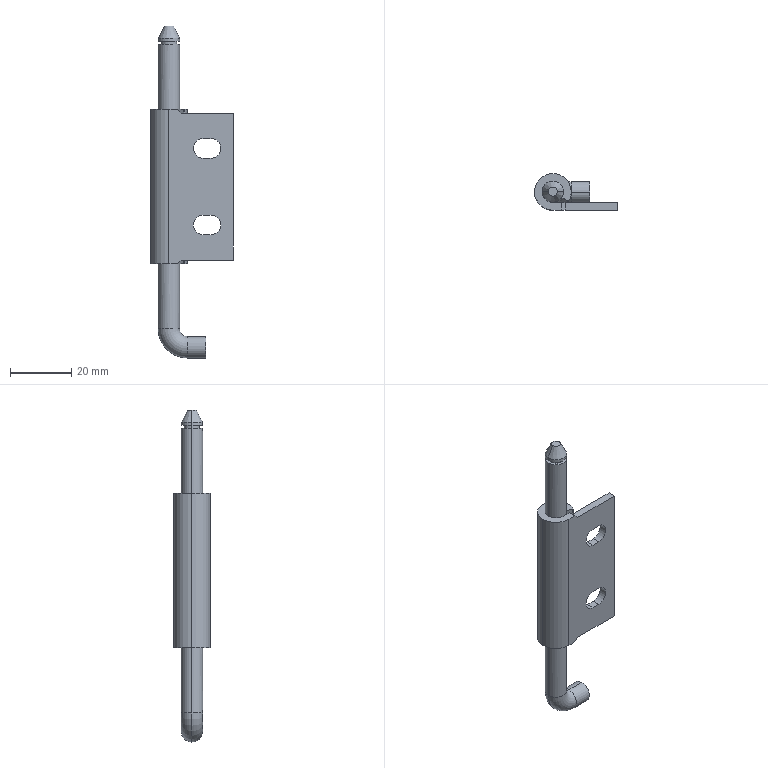Part | NX | features BREP 1 | 1 solid | 42 faces | box 27.1 x 12 x 108.5 mm | volume 9783 mm3 | plane 22 | cylinder 16 | cone 2 | torus 2 | commonest cylinder face diameters 7 x7 6.4 x4 12 x3 5 x2
STEP:
#1=CARTESIAN_POINT('',(-1.5,0.,52.5));
#2=VERTEX_POINT('',#1);
#3=CARTESIAN_POINT('',(1.5,0.,52.5));
#4=VERTEX_POINT('',#3);
#5=CARTESIAN_POINT('',(0.,0.,52.5));
#6=DIRECTION('',(0.,0.,-1.));
#7=DIRECTION('',(-1.,0.,0.));
#8=AXIS2_PLACEMENT_3D('',#5,#6,#7);
#9=CIRCLE('',#8,1.5);
#10=EDGE_CURVE('',#2,#4,#9,.T.);
#11=ORIENTED_EDGE('',*,*,#10,.F.);
#12=CARTESIAN_POINT('',(0.,0.,52.5));
#13=DIRECTION('',(0.,0.,-1.));
#14=DIRECTION('',(-1.,0.,0.));
#15=AXIS2_PLACEMENT_3D('',#12,#13,#14);
#16=CIRCLE('',#15,1.5);
#17=EDGE_CURVE('',#4,#2,#16,.T.);
#18=ORIENTED_EDGE('',*,*,#17,.F.);
#19=EDGE_LOOP('',(#11,#18));
#20=FACE_BOUND('',#19,.T.);
#21=CARTESIAN_POINT('',(0.,0.,52.5));
#22=DIRECTION('',(0.,0.,-1.));
#23=DIRECTION('',(-1.,0.,0.));
#24=AXIS2_PLACEMENT_3D('',#21,#22,#23);
#25=PLANE('',#24);
#26=ADVANCED_FACE('',(#20),#25,.F.);
#27=CARTESIAN_POINT('',(3.5,0.,48.5));
#28=VERTEX_POINT('',#27);
#29=CARTESIAN_POINT('',(1.5,0.,52.5));
#30=DIRECTION('',(0.4472,0.,-0.8944));
#31=VECTOR('',#30,1000.);
#32=LINE('',#29,#31);
#33=EDGE_CURVE('',#4,#28,#32,.T.);
#34=ORIENTED_EDGE('',*,*,#33,.F.);
#35=ORIENTED_EDGE('',*,*,#17,.T.);
#36=CARTESIAN_POINT('',(-3.5,0.,48.5));
#37=VERTEX_POINT('',#36);
#38=CARTESIAN_POINT('',(-1.5,0.,52.5));
#39=DIRECTION('',(-0.4472,0.,-0.8944));
#40=VECTOR('',#39,1000.);
#41=LINE('',#38,#40);
#42=EDGE_CURVE('',#2,#37,#41,.T.);
#43=ORIENTED_EDGE('',*,*,#42,.T.);
#44=CARTESIAN_POINT('',(0.,0.,48.5));
#45=DIRECTION('',(0.,0.,-1.));
#46=DIRECTION('',(-1.,0.,0.));
#47=AXIS2_PLACEMENT_3D('',#44,#45,#46);
#48=CIRCLE('',#47,3.5);
#49=EDGE_CURVE('',#28,#37,#48,.T.);
#50=ORIENTED_EDGE('',*,*,#49,.F.);
#51=EDGE_LOOP('',(#34,#35,#43,#50));
#52=FACE_BOUND('',#51,.T.);
#53=CARTESIAN_POINT('',(0.,0.,52.5));
#54=DIRECTION('',(0.,0.,-1.));
#55=DIRECTION('',(-1.,0.,0.));
#56=AXIS2_PLACEMENT_3D('',#53,#54,#55);
#57=CONICAL_SURFACE('',#56,1.5,0.4636);
#58=ADVANCED_FACE('',(#52),#57,.T.);
#59=CARTESIAN_POINT('',(3.5,0.,47.5));
#60=VERTEX_POINT('',#59);
#61=CARTESIAN_POINT('',(3.5,0.,-46.5));
#62=DIRECTION('',(0.,0.,-1.));
#63=VECTOR('',#62,1000.);
#64=LINE('',#61,#63);
#65=EDGE_CURVE('',#28,#60,#64,.T.);
#66=ORIENTED_EDGE('',*,*,#65,.F.);
#67=ORIENTED_EDGE('',*,*,#49,.T.);
#68=CARTESIAN_POINT('',(-3.5,0.,47.5));
#69=VERTEX_POINT('',#68);
#70=CARTESIAN_POINT('',(-3.5,0.,-46.5));
#71=DIRECTION('',(0.,0.,-1.));
#72=VECTOR('',#71,1000.);
#73=LINE('',#70,#72);
#74=EDGE_CURVE('',#37,#69,#73,.T.);
#75=ORIENTED_EDGE('',*,*,#74,.T.);
#76=CARTESIAN_POINT('',(0.,0.,47.5));
#77=DIRECTION('',(0.,0.,-1.));
#78=DIRECTION('',(-1.,0.,0.));
#79=AXIS2_PLACEMENT_3D('',#76,#77,#78);
#80=CIRCLE('',#79,3.5);
#81=EDGE_CURVE('',#60,#69,#80,.T.);
#82=ORIENTED_EDGE('',*,*,#81,.F.);
#83=EDGE_LOOP('',(#66,#67,#75,#82));
#84=FACE_BOUND('',#83,.T.);
#85=CARTESIAN_POINT('',(0.,0.,-46.5));
#86=DIRECTION('',(0.,0.,-1.));
#87=DIRECTION('',(-1.,0.,0.));
#88=AXIS2_PLACEMENT_3D('',#85,#86,#87);
#89=CYLINDRICAL_SURFACE('',#88,3.5);
#90=ADVANCED_FACE('',(#84),#89,.T.);
#91=CARTESIAN_POINT('',(0.,0.,47.5));
#92=DIRECTION('',(0.,0.,-1.));
#93=DIRECTION('',(-1.,0.,0.));
#94=AXIS2_PLACEMENT_3D('',#91,#92,#93);
#95=CIRCLE('',#94,3.5);
#96=EDGE_CURVE('',#69,#60,#95,.T.);
#97=ORIENTED_EDGE('',*,*,#96,.T.);
#98=ORIENTED_EDGE('',*,*,#81,.T.);
#99=EDGE_LOOP('',(#97,#98));
#100=FACE_BOUND('',#99,.T.);
#101=CARTESIAN_POINT('',(-2.5,0.,47.5));
#102=VERTEX_POINT('',#101);
#103=CARTESIAN_POINT('',(2.5,0.,47.5));
#104=VERTEX_POINT('',#103);
#105=CARTESIAN_POINT('',(0.,0.,47.5));
#106=DIRECTION('',(0.,0.,-1.));
#107=DIRECTION('',(-1.,0.,0.));
#108=AXIS2_PLACEMENT_3D('',#105,#106,#107);
#109=CIRCLE('',#108,2.5);
#110=EDGE_CURVE('',#102,#104,#109,.T.);
#111=ORIENTED_EDGE('',*,*,#110,.F.);
#112=CARTESIAN_POINT('',(0.,0.,47.5));
#113=DIRECTION('',(0.,0.,-1.));
#114=DIRECTION('',(-1.,0.,0.));
#115=AXIS2_PLACEMENT_3D('',#112,#113,#114);
#116=CIRCLE('',#115,2.5);
#117=EDGE_CURVE('',#104,#102,#116,.T.);
#118=ORIENTED_EDGE('',*,*,#117,.F.);
#119=EDGE_LOOP('',(#111,#118));
#120=FACE_BOUND('',#119,.T.);
#121=CARTESIAN_POINT('',(-3.5,0.,47.5));
#122=DIRECTION('',(0.,0.,1.));
#123=DIRECTION('',(1.,0.,0.));
#124=AXIS2_PLACEMENT_3D('',#121,#122,#123);
#125=PLANE('',#124);
#126=ADVANCED_FACE('',(#100,#120),#125,.F.);
#127=CARTESIAN_POINT('',(12.,0.,-49.));
#128=VERTEX_POINT('',#127);
#129=CARTESIAN_POINT('',(12.,0.,-56.));
#130=VERTEX_POINT('',#129);
#131=CARTESIAN_POINT('',(12.,0.,-52.5));
#132=DIRECTION('',(1.,0.,0.));
#133=DIRECTION('',(0.,0.,-1.));
#134=AXIS2_PLACEMENT_3D('',#131,#132,#133);
#135=CIRCLE('',#134,3.5);
#136=EDGE_CURVE('',#128,#130,#135,.T.);
#137=ORIENTED_EDGE('',*,*,#136,.T.);
#138=CARTESIAN_POINT('',(12.,0.,-52.5));
#139=DIRECTION('',(1.,0.,0.));
#140=DIRECTION('',(0.,0.,-1.));
#141=AXIS2_PLACEMENT_3D('',#138,#139,#140);
#142=CIRCLE('',#141,3.5);
#143=EDGE_CURVE('',#130,#128,#142,.T.);
#144=ORIENTED_EDGE('',*,*,#143,.T.);
#145=EDGE_LOOP('',(#137,#144));
#146=FACE_BOUND('',#145,.T.);
#147=CARTESIAN_POINT('',(12.,0.,-52.5));
#148=DIRECTION('',(1.,0.,0.));
#149=DIRECTION('',(0.,0.,-1.));
#150=AXIS2_PLACEMENT_3D('',#147,#148,#149);
#151=PLANE('',#150);
#152=ADVANCED_FACE('',(#146),#151,.T.);
#153=CARTESIAN_POINT('',(21.1,-6.,24.));
#154=VERTEX_POINT('',#153);
#155=CARTESIAN_POINT('',(21.1,-6.,-24.));
#156=VERTEX_POINT('',#155);
#157=CARTESIAN_POINT('',(21.1,-6.,24.));
#158=DIRECTION('',(0.,0.,-1.));
#159=VECTOR('',#158,1000.);
#160=LINE('',#157,#159);
#161=EDGE_CURVE('',#154,#156,#160,.T.);
#162=ORIENTED_EDGE('',*,*,#161,.T.);
#163=CARTESIAN_POINT('',(21.1,-3.5,-24.));
#164=VERTEX_POINT('',#163);
#165=CARTESIAN_POINT('',(21.1,-6.,-24.));
#166=DIRECTION('',(0.,1.,0.));
#167=VECTOR('',#166,1000.);
#168=LINE('',#165,#167);
#169=EDGE_CURVE('',#156,#164,#168,.T.);
#170=ORIENTED_EDGE('',*,*,#169,.T.);
#171=CARTESIAN_POINT('',(21.1,-3.5,24.));
#172=VERTEX_POINT('',#171);
#173=CARTESIAN_POINT('',(21.1,-3.5,24.));
#174=DIRECTION('',(0.,0.,-1.));
#175=VECTOR('',#174,1000.);
#176=LINE('',#173,#175);
#177=EDGE_CURVE('',#172,#164,#176,.T.);
#178=ORIENTED_EDGE('',*,*,#177,.F.);
#179=CARTESIAN_POINT('',(21.1,-3.5,24.));
#180=DIRECTION('',(0.,-1.,0.));
#181=VECTOR('',#180,1000.);
#182=LINE('',#179,#181);
#183=EDGE_CURVE('',#172,#154,#182,.T.);
#184=ORIENTED_EDGE('',*,*,#183,.T.);
#185=EDGE_LOOP('',(#162,#170,#178,#184));
#186=FACE_BOUND('',#185,.T.);
#187=CARTESIAN_POINT('',(21.1,-6.,25.25));
#188=DIRECTION('',(-1.,0.,0.));
#189=DIRECTION('',(0.,0.,1.));
#190=AXIS2_PLACEMENT_3D('',#187,#188,#189);
#191=PLANE('',#190);
#192=ADVANCED_FACE('',(#186),#191,.F.);
#193=ORIENTED_EDGE('',*,*,#183,.F.);
#194=CARTESIAN_POINT('',(4.,-3.5,24.));
#195=VERTEX_POINT('',#194);
#196=CARTESIAN_POINT('',(4.,-3.5,24.));
#197=DIRECTION('',(1.,0.,0.));
#198=VECTOR('',#197,1000.);
#199=LINE('',#196,#198);
#200=EDGE_CURVE('',#195,#172,#199,.T.);
#201=ORIENTED_EDGE('',*,*,#200,.F.);
#202=CARTESIAN_POINT('',(4.,-6.,24.));
#203=VERTEX_POINT('',#202);
#204=CARTESIAN_POINT('',(4.,-3.5,24.));
#205=DIRECTION('',(0.,-1.,0.));
#206=VECTOR('',#205,1000.);
#207=LINE('',#204,#206);
#208=EDGE_CURVE('',#195,#203,#207,.T.);
#209=ORIENTED_EDGE('',*,*,#208,.T.);
#210=CARTESIAN_POINT('',(21.1,-6.,24.));
#211=DIRECTION('',(-1.,0.,0.));
#212=VECTOR('',#211,1000.);
#213=LINE('',#210,#212);
#214=EDGE_CURVE('',#154,#203,#213,.T.);
#215=ORIENTED_EDGE('',*,*,#214,.F.);
#216=EDGE_LOOP('',(#193,#201,#209,#215));
#217=FACE_BOUND('',#216,.T.);
#218=CARTESIAN_POINT('',(4.,-3.,24.));
#219=DIRECTION('',(0.,0.,-1.));
#220=DIRECTION('',(-1.,0.,0.));
#221=AXIS2_PLACEMENT_3D('',#218,#219,#220);
#222=PLANE('',#221);
#223=ADVANCED_FACE('',(#217),#222,.F.);
#224=CARTESIAN_POINT('',(4.,-3.5,-24.));
#225=VERTEX_POINT('',#224);
#226=CARTESIAN_POINT('',(4.,-6.,-24.));
#227=VERTEX_POINT('',#226);
#228=CARTESIAN_POINT('',(4.,-3.5,-24.));
#229=DIRECTION('',(0.,-1.,0.));
#230=VECTOR('',#229,1000.);
#231=LINE('',#228,#230);
#232=EDGE_CURVE('',#225,#227,#231,.T.);
#233=ORIENTED_EDGE('',*,*,#232,.F.);
#234=CARTESIAN_POINT('',(21.1,-3.5,-24.));
#235=DIRECTION('',(-1.,0.,0.));
#236=VECTOR('',#235,1000.);
#237=LINE('',#234,#236);
#238=EDGE_CURVE('',#164,#225,#237,.T.);
#239=ORIENTED_EDGE('',*,*,#238,.F.);
#240=ORIENTED_EDGE('',*,*,#169,.F.);
#241=CARTESIAN_POINT('',(4.,-6.,-24.));
#242=DIRECTION('',(1.,0.,0.));
#243=VECTOR('',#242,1000.);
#244=LINE('',#241,#243);
#245=EDGE_CURVE('',#227,#156,#244,.T.);
#246=ORIENTED_EDGE('',*,*,#245,.F.);
#247=EDGE_LOOP('',(#233,#239,#240,#246));
#248=FACE_BOUND('',#247,.T.);
#249=CARTESIAN_POINT('',(22.9,-3.,-24.));
#250=DIRECTION('',(0.,0.,1.));
#251=DIRECTION('',(1.,0.,0.));
#252=AXIS2_PLACEMENT_3D('',#249,#250,#251);
#253=PLANE('',#252);
#254=ADVANCED_FACE('',(#248),#253,.F.);
#255=CARTESIAN_POINT('',(11.2,-6.,15.7));
#256=VERTEX_POINT('',#255);
#257=CARTESIAN_POINT('',(11.2,-6.,9.3));
#258=VERTEX_POINT('',#257);
#259=CARTESIAN_POINT('',(11.2,-6.,12.5));
#260=DIRECTION('',(0.,-1.,0.));
#261=DIRECTION('',(0.,0.,1.));
#262=AXIS2_PLACEMENT_3D('',#259,#260,#261);
#263=CIRCLE('',#262,3.2);
#264=EDGE_CURVE('',#256,#258,#263,.T.);
#265=ORIENTED_EDGE('',*,*,#264,.T.);
#266=CARTESIAN_POINT('',(11.2,-3.5,9.3));
#267=VERTEX_POINT('',#266);
#268=CARTESIAN_POINT('',(11.2,-3.5,9.3));
#269=DIRECTION('',(0.,-1.,0.));
#270=VECTOR('',#269,1000.);
#271=LINE('',#268,#270);
#272=EDGE_CURVE('',#267,#258,#271,.T.);
#273=ORIENTED_EDGE('',*,*,#272,.F.);
#274=CARTESIAN_POINT('',(11.2,-3.5,15.7));
#275=VERTEX_POINT('',#274);
#276=CARTESIAN_POINT('',(11.2,-3.5,12.5));
#277=DIRECTION('',(0.,1.,0.));
#278=DIRECTION('',(0.,0.,-1.));
#279=AXIS2_PLACEMENT_3D('',#276,#277,#278);
#280=CIRCLE('',#279,3.2);
#281=EDGE_CURVE('',#267,#275,#280,.T.);
#282=ORIENTED_EDGE('',*,*,#281,.T.);
#283=CARTESIAN_POINT('',(11.2,-3.5,15.7));
#284=DIRECTION('',(0.,-1.,0.));
#285=VECTOR('',#284,1000.);
#286=LINE('',#283,#285);
#287=EDGE_CURVE('',#275,#256,#286,.T.);
#288=ORIENTED_EDGE('',*,*,#287,.T.);
#289=EDGE_LOOP('',(#265,#273,#282,#288));
#290=FACE_BOUND('',#289,.T.);
#291=CARTESIAN_POINT('',(11.2,-3.,12.5));
#292=DIRECTION('',(0.,-1.,0.));
#293=DIRECTION('',(0.,0.,-1.));
#294=AXIS2_PLACEMENT_3D('',#291,#292,#293);
#295=CYLINDRICAL_SURFACE('',#294,3.2);
#296=ADVANCED_FACE('',(#290),#295,.F.);
#297=CARTESIAN_POINT('',(13.8,-6.,15.7));
#298=VERTEX_POINT('',#297);
#299=CARTESIAN_POINT('',(13.8,-6.,15.7));
#300=DIRECTION('',(-1.,0.,0.));
#301=VECTOR('',#300,1000.);
#302=LINE('',#299,#301);
#303=EDGE_CURVE('',#298,#256,#302,.T.);
#304=ORIENTED_EDGE('',*,*,#303,.T.);
#305=ORIENTED_EDGE('',*,*,#287,.F.);
#306=CARTESIAN_POINT('',(13.8,-3.5,15.7));
#307=VERTEX_POINT('',#306);
#308=CARTESIAN_POINT('',(11.2,-3.5,15.7));
#309=DIRECTION('',(1.,0.,0.));
#310=VECTOR('',#309,1000.);
#311=LINE('',#308,#310);
#312=EDGE_CURVE('',#275,#307,#311,.T.);
#313=ORIENTED_EDGE('',*,*,#312,.T.);
#314=CARTESIAN_POINT('',(13.8,-3.5,15.7));
#315=DIRECTION('',(0.,-1.,0.));
#316=VECTOR('',#315,1000.);
#317=LINE('',#314,#316);
#318=EDGE_CURVE('',#307,#298,#317,.T.);
#319=ORIENTED_EDGE('',*,*,#318,.T.);
#320=EDGE_LOOP('',(#304,#305,#313,#319));
#321=FACE_BOUND('',#320,.T.);
#322=CARTESIAN_POINT('',(11.2,-3.,15.7));
#323=DIRECTION('',(0.,0.,-1.));
#324=DIRECTION('',(-1.,0.,0.));
#325=AXIS2_PLACEMENT_3D('',#322,#323,#324);
#326=PLANE('',#325);
#327=ADVANCED_FACE('',(#321),#326,.T.);
#328=CARTESIAN_POINT('',(13.8,-6.,9.3));
#329=VERTEX_POINT('',#328);
#330=CARTESIAN_POINT('',(13.8,-6.,12.5));
#331=DIRECTION('',(0.,-1.,0.));
#332=DIRECTION('',(0.,0.,-1.));
#333=AXIS2_PLACEMENT_3D('',#330,#331,#332);
#334=CIRCLE('',#333,3.2);
#335=EDGE_CURVE('',#329,#298,#334,.T.);
#336=ORIENTED_EDGE('',*,*,#335,.T.);
#337=ORIENTED_EDGE('',*,*,#318,.F.);
#338=CARTESIAN_POINT('',(13.8,-3.5,9.3));
#339=VERTEX_POINT('',#338);
#340=CARTESIAN_POINT('',(13.8,-3.5,12.5));
#341=DIRECTION('',(0.,1.,0.));
#342=DIRECTION('',(0.,0.,1.));
#343=AXIS2_PLACEMENT_3D('',#340,#341,#342);
#344=CIRCLE('',#343,3.2);
#345=EDGE_CURVE('',#307,#339,#344,.T.);
#346=ORIENTED_EDGE('',*,*,#345,.T.);
#347=CARTESIAN_POINT('',(13.8,-3.5,9.3));
#348=DIRECTION('',(0.,-1.,0.));
#349=VECTOR('',#348,1000.);
#350=LINE('',#347,#349);
#351=EDGE_CURVE('',#339,#329,#350,.T.);
#352=ORIENTED_EDGE('',*,*,#351,.T.);
#353=EDGE_LOOP('',(#336,#337,#346,#352));
#354=FACE_BOUND('',#353,.T.);
#355=CARTESIAN_POINT('',(13.8,-3.,12.5));
#356=DIRECTION('',(0.,-1.,0.));
#357=DIRECTION('',(0.,0.,-1.));
#358=AXIS2_PLACEMENT_3D('',#355,#356,#357);
#359=CYLINDRICAL_SURFACE('',#358,3.2);
#360=ADVANCED_FACE('',(#354),#359,.F.);
#361=CARTESIAN_POINT('',(11.2,-6.,9.3));
#362=DIRECTION('',(1.,0.,0.));
#363=VECTOR('',#362,1000.);
#364=LINE('',#361,#363);
#365=EDGE_CURVE('',#258,#329,#364,.T.);
#366=ORIENTED_EDGE('',*,*,#365,.T.);
#367=ORIENTED_EDGE('',*,*,#351,.F.);
#368=CARTESIAN_POINT('',(13.8,-3.5,9.3));
#369=DIRECTION('',(-1.,0.,0.));
#370=VECTOR('',#369,1000.);
#371=LINE('',#368,#370);
#372=EDGE_CURVE('',#339,#267,#371,.T.);
#373=ORIENTED_EDGE('',*,*,#372,.T.);
#374=ORIENTED_EDGE('',*,*,#272,.T.);
#375=EDGE_LOOP('',(#366,#367,#373,#374));
#376=FACE_BOUND('',#375,.T.);
#377=CARTESIAN_POINT('',(13.8,-3.,9.3));
#378=DIRECTION('',(0.,0.,1.));
#379=DIRECTION('',(1.,0.,0.));
#380=AXIS2_PLACEMENT_3D('',#377,#378,#379);
#381=PLANE('',#380);
#382=ADVANCED_FACE('',(#376),#381,.T.);
#383=CARTESIAN_POINT('',(11.2,-6.,-9.3));
#384=VERTEX_POINT('',#383);
#385=CARTESIAN_POINT('',(11.2,-6.,-15.7));
#386=VERTEX_POINT('',#385);
#387=CARTESIAN_POINT('',(11.2,-6.,-12.5));
#388=DIRECTION('',(0.,-1.,0.));
#389=DIRECTION('',(0.,0.,1.));
#390=AXIS2_PLACEMENT_3D('',#387,#388,#389);
#391=CIRCLE('',#390,3.2);
#392=EDGE_CURVE('',#384,#386,#391,.T.);
#393=ORIENTED_EDGE('',*,*,#392,.T.);
#394=CARTESIAN_POINT('',(11.2,-3.5,-15.7));
#395=VERTEX_POINT('',#394);
#396=CARTESIAN_POINT('',(11.2,-3.5,-15.7));
#397=DIRECTION('',(0.,-1.,0.));
#398=VECTOR('',#397,1000.);
#399=LINE('',#396,#398);
#400=EDGE_CURVE('',#395,#386,#399,.T.);
#401=ORIENTED_EDGE('',*,*,#400,.F.);
#402=CARTESIAN_POINT('',(11.2,-3.5,-9.3));
#403=VERTEX_POINT('',#402);
#404=CARTESIAN_POINT('',(11.2,-3.5,-12.5));
#405=DIRECTION('',(0.,1.,0.));
#406=DIRECTION('',(0.,0.,-1.));
#407=AXIS2_PLACEMENT_3D('',#404,#405,#406);
#408=CIRCLE('',#407,3.2);
#409=EDGE_CURVE('',#395,#403,#408,.T.);
#410=ORIENTED_EDGE('',*,*,#409,.T.);
#411=CARTESIAN_POINT('',(11.2,-3.5,-9.3));
#412=DIRECTION('',(0.,-1.,0.));
#413=VECTOR('',#412,1000.);
#414=LINE('',#411,#413);
#415=EDGE_CURVE('',#403,#384,#414,.T.);
#416=ORIENTED_EDGE('',*,*,#415,.T.);
#417=EDGE_LOOP('',(#393,#401,#410,#416));
#418=FACE_BOUND('',#417,.T.);
#419=CARTESIAN_POINT('',(11.2,-3.,-12.5));
#420=DIRECTION('',(0.,-1.,0.));
#421=DIRECTION('',(0.,0.,-1.));
#422=AXIS2_PLACEMENT_3D('',#419,#420,#421);
#423=CYLINDRICAL_SURFACE('',#422,3.2);
#424=ADVANCED_FACE('',(#418),#423,.F.);
#425=CARTESIAN_POINT('',(13.8,-6.,-9.3));
#426=VERTEX_POINT('',#425);
#427=CARTESIAN_POINT('',(13.8,-6.,-9.3));
#428=DIRECTION('',(-1.,0.,0.));
#429=VECTOR('',#428,1000.);
#430=LINE('',#427,#429);
#431=EDGE_CURVE('',#426,#384,#430,.T.);
#432=ORIENTED_EDGE('',*,*,#431,.T.);
#433=ORIENTED_EDGE('',*,*,#415,.F.);
#434=CARTESIAN_POINT('',(13.8,-3.5,-9.3));
#435=VERTEX_POINT('',#434);
#436=CARTESIAN_POINT('',(11.2,-3.5,-9.3));
#437=DIRECTION('',(1.,0.,0.));
#438=VECTOR('',#437,1000.);
#439=LINE('',#436,#438);
#440=EDGE_CURVE('',#403,#435,#439,.T.);
#441=ORIENTED_EDGE('',*,*,#440,.T.);
#442=CARTESIAN_POINT('',(13.8,-3.5,-9.3));
#443=DIRECTION('',(0.,-1.,0.));
#444=VECTOR('',#443,1000.);
#445=LINE('',#442,#444);
#446=EDGE_CURVE('',#435,#426,#445,.T.);
#447=ORIENTED_EDGE('',*,*,#446,.T.);
#448=EDGE_LOOP('',(#432,#433,#441,#447));
#449=FACE_BOUND('',#448,.T.);
#450=CARTESIAN_POINT('',(11.2,-3.,-9.3));
#451=DIRECTION('',(0.,0.,-1.));
#452=DIRECTION('',(-1.,0.,0.));
#453=AXIS2_PLACEMENT_3D('',#450,#451,#452);
#454=PLANE('',#453);
#455=ADVANCED_FACE('',(#449),#454,.T.);
#456=CARTESIAN_POINT('',(13.8,-6.,-15.7));
#457=VERTEX_POINT('',#456);
#458=CARTESIAN_POINT('',(13.8,-6.,-12.5));
#459=DIRECTION('',(0.,-1.,0.));
#460=DIRECTION('',(0.,0.,-1.));
#461=AXIS2_PLACEMENT_3D('',#458,#459,#460);
#462=CIRCLE('',#461,3.2);
#463=EDGE_CURVE('',#457,#426,#462,.T.);
#464=ORIENTED_EDGE('',*,*,#463,.T.);
#465=ORIENTED_EDGE('',*,*,#446,.F.);
#466=CARTESIAN_POINT('',(13.8,-3.5,-15.7));
#467=VERTEX_POINT('',#466);
#468=CARTESIAN_POINT('',(13.8,-3.5,-12.5));
#469=DIRECTION('',(0.,1.,0.));
#470=DIRECTION('',(0.,0.,1.));
#471=AXIS2_PLACEMENT_3D('',#468,#469,#470);
#472=CIRCLE('',#471,3.2);
#473=EDGE_CURVE('',#435,#467,#472,.T.);
#474=ORIENTED_EDGE('',*,*,#473,.T.);
#475=CARTESIAN_POINT('',(13.8,-3.5,-15.7));
#476=DIRECTION('',(0.,-1.,0.));
#477=VECTOR('',#476,1000.);
#478=LINE('',#475,#477);
#479=EDGE_CURVE('',#467,#457,#478,.T.);
#480=ORIENTED_EDGE('',*,*,#479,.T.);
#481=EDGE_LOOP('',(#464,#465,#474,#480));
#482=FACE_BOUND('',#481,.T.);
#483=CARTESIAN_POINT('',(13.8,-3.,-12.5));
#484=DIRECTION('',(0.,-1.,0.));
#485=DIRECTION('',(0.,0.,-1.));
#486=AXIS2_PLACEMENT_3D('',#483,#484,#485);
#487=CYLINDRICAL_SURFACE('',#486,3.2);
#488=ADVANCED_FACE('',(#482),#487,.F.);
#489=CARTESIAN_POINT('',(11.2,-6.,-15.7));
#490=DIRECTION('',(1.,0.,0.));
#491=VECTOR('',#490,1000.);
#492=LINE('',#489,#491);
#493=EDGE_CURVE('',#386,#457,#492,.T.);
#494=ORIENTED_EDGE('',*,*,#493,.T.);
#495=ORIENTED_EDGE('',*,*,#479,.F.);
#496=CARTESIAN_POINT('',(13.8,-3.5,-15.7));
#497=DIRECTION('',(-1.,0.,0.));
#498=VECTOR('',#497,1000.);
#499=LINE('',#496,#498);
#500=EDGE_CURVE('',#467,#395,#499,.T.);
#501=ORIENTED_EDGE('',*,*,#500,.T.);
#502=ORIENTED_EDGE('',*,*,#400,.T.);
#503=EDGE_LOOP('',(#494,#495,#501,#502));
#504=FACE_BOUND('',#503,.T.);
#505=CARTESIAN_POINT('',(13.8,-3.,-15.7));
#506=DIRECTION('',(0.,0.,1.));
#507=DIRECTION('',(1.,0.,0.));
#508=AXIS2_PLACEMENT_3D('',#505,#506,#507);
#509=PLANE('',#508);
#510=ADVANCED_FACE('',(#504),#509,.T.);
#511=CARTESIAN_POINT('',(2.5,0.,46.5));
#512=VERTEX_POINT('',#511);
#513=CARTESIAN_POINT('',(2.5,0.,-46.5));
#514=DIRECTION('',(0.,0.,-1.));
#515=VECTOR('',#514,1000.);
#516=LINE('',#513,#515);
#517=EDGE_CURVE('',#104,#512,#516,.T.);
#518=ORIENTED_EDGE('',*,*,#517,.F.);
#519=ORIENTED_EDGE('',*,*,#117,.T.);
#520=CARTESIAN_POINT('',(-2.5,0.,46.5));
#521=VERTEX_POINT('',#520);
#522=CARTESIAN_POINT('',(-2.5,0.,-46.5));
#523=DIRECTION('',(0.,0.,-1.));
#524=VECTOR('',#523,1000.);
#525=LINE('',#522,#524);
#526=EDGE_CURVE('',#102,#521,#525,.T.);
#527=ORIENTED_EDGE('',*,*,#526,.T.);
#528=CARTESIAN_POINT('',(0.,0.,46.5));
#529=DIRECTION('',(0.,0.,-1.));
#530=DIRECTION('',(-1.,0.,0.));
#531=AXIS2_PLACEMENT_3D('',#528,#529,#530);
#532=CIRCLE('',#531,2.5);
#533=EDGE_CURVE('',#512,#521,#532,.T.);
#534=ORIENTED_EDGE('',*,*,#533,.F.);
#535=EDGE_LOOP('',(#518,#519,#527,#534));
#536=FACE_BOUND('',#535,.T.);
#537=CARTESIAN_POINT('',(0.,0.,-46.5));
#538=DIRECTION('',(0.,0.,-1.));
#539=DIRECTION('',(-1.,0.,0.));
#540=AXIS2_PLACEMENT_3D('',#537,#538,#539);
#541=CYLINDRICAL_SURFACE('',#540,2.5);
#542=ADVANCED_FACE('',(#536),#541,.T.);
#543=CARTESIAN_POINT('',(6.,0.,-56.));
#544=VERTEX_POINT('',#543);
#545=CARTESIAN_POINT('',(12.,0.,-56.));
#546=DIRECTION('',(-1.,0.,0.));
#547=VECTOR('',#546,1000.);
#548=LINE('',#545,#547);
#549=EDGE_CURVE('',#544,#130,#548,.F.);
#550=ORIENTED_EDGE('',*,*,#549,.T.);
#551=ORIENTED_EDGE('',*,*,#136,.F.);
#552=CARTESIAN_POINT('',(6.,0.,-49.));
#553=VERTEX_POINT('',#552);
#554=CARTESIAN_POINT('',(12.,0.,-49.));
#555=DIRECTION('',(-1.,0.,0.));
#556=VECTOR('',#555,1000.);
#557=LINE('',#554,#556);
#558=EDGE_CURVE('',#553,#128,#557,.F.);
#559=ORIENTED_EDGE('',*,*,#558,.F.);
#560=CARTESIAN_POINT('',(6.,0.,-52.5));
#561=DIRECTION('',(1.,0.,0.));
#562=DIRECTION('',(0.,0.,-1.));
#563=AXIS2_PLACEMENT_3D('',#560,#561,#562);
#564=CIRCLE('',#563,3.5);
#565=EDGE_CURVE('',#553,#544,#564,.T.);
#566=ORIENTED_EDGE('',*,*,#565,.T.);
#567=EDGE_LOOP('',(#550,#551,#559,#566));
#568=FACE_BOUND('',#567,.T.);
#569=CARTESIAN_POINT('',(12.,0.,-52.5));
#570=DIRECTION('',(-1.,0.,0.));
#571=DIRECTION('',(0.,0.,1.));
#572=AXIS2_PLACEMENT_3D('',#569,#570,#571);
#573=CYLINDRICAL_SURFACE('',#572,3.5);
#574=ADVANCED_FACE('',(#568),#573,.T.);
#575=ORIENTED_EDGE('',*,*,#208,.F.);
#576=CARTESIAN_POINT('',(2.75,-3.5,25.25));
#577=VERTEX_POINT('',#576);
#578=CARTESIAN_POINT('',(2.75,-3.5,25.25));
#579=DIRECTION('',(0.7071,0.,-0.7071));
#580=VECTOR('',#579,1000.);
#581=LINE('',#578,#580);
#582=EDGE_CURVE('',#577,#195,#581,.T.);
#583=ORIENTED_EDGE('',*,*,#582,.F.);
#584=CARTESIAN_POINT('',(2.75,-6.,25.25));
#585=VERTEX_POINT('',#584);
#586=CARTESIAN_POINT('',(2.75,-3.5,25.25));
#587=DIRECTION('',(0.,-1.,0.));
#588=VECTOR('',#587,1000.);
#589=LINE('',#586,#588);
#590=EDGE_CURVE('',#577,#585,#589,.T.);
#591=ORIENTED_EDGE('',*,*,#590,.T.);
#592=CARTESIAN_POINT('',(4.,-6.,24.));
#593=DIRECTION('',(-0.7071,0.,0.7071));
#594=VECTOR('',#593,1000.);
#595=LINE('',#592,#594);
#596=EDGE_CURVE('',#203,#585,#595,.T.);
#597=ORIENTED_EDGE('',*,*,#596,.F.);
#598=EDGE_LOOP('',(#575,#583,#591,#597));
#599=FACE_BOUND('',#598,.T.);
#600=CARTESIAN_POINT('',(2.75,-3.,25.25));
#601=DIRECTION('',(-0.7071,0.,-0.7071));
#602=DIRECTION('',(-0.7071,0.,0.7071));
#603=AXIS2_PLACEMENT_3D('',#600,#601,#602);
#604=PLANE('',#603);
#605=ADVANCED_FACE('',(#599),#604,.F.);
#606=CARTESIAN_POINT('',(0.,-6.,-25.25));
#607=VERTEX_POINT('',#606);
#608=CARTESIAN_POINT('',(2.75,-6.,-25.25));
#609=VERTEX_POINT('',#608);
#610=CARTESIAN_POINT('',(0.,-6.,-25.25));
#611=DIRECTION('',(1.,0.,0.));
#612=VECTOR('',#611,1000.);
#613=LINE('',#610,#612);
#614=EDGE_CURVE('',#607,#609,#613,.T.);
#615=ORIENTED_EDGE('',*,*,#614,.T.);
#616=CARTESIAN_POINT('',(2.75,-6.,-25.25));
#617=DIRECTION('',(0.7071,0.,0.7071));
#618=VECTOR('',#617,1000.);
#619=LINE('',#616,#618);
#620=EDGE_CURVE('',#609,#227,#619,.T.);
#621=ORIENTED_EDGE('',*,*,#620,.T.);
#622=ORIENTED_EDGE('',*,*,#245,.T.);
#623=ORIENTED_EDGE('',*,*,#161,.F.);
#624=ORIENTED_EDGE('',*,*,#214,.T.);
#625=ORIENTED_EDGE('',*,*,#596,.T.);
#626=CARTESIAN_POINT('',(0.,-6.,25.25));
#627=VERTEX_POINT('',#626);
#628=CARTESIAN_POINT('',(0.,-6.,25.25));
#629=DIRECTION('',(1.,0.,0.));
#630=VECTOR('',#629,1000.);
#631=LINE('',#628,#630);
#632=EDGE_CURVE('',#627,#585,#631,.T.);
#633=ORIENTED_EDGE('',*,*,#632,.F.);
#634=CARTESIAN_POINT('',(0.,-6.,25.25));
#635=DIRECTION('',(0.,0.,-1.));
#636=VECTOR('',#635,1000.);
#637=LINE('',#634,#636);
#638=EDGE_CURVE('',#627,#607,#637,.T.);
#639=ORIENTED_EDGE('',*,*,#638,.T.);
#640=EDGE_LOOP('',(#615,#621,#622,#623,#624,#625,#633,#639));
#641=FACE_BOUND('',#640,.T.);
#642=ORIENTED_EDGE('',*,*,#365,.F.);
#643=ORIENTED_EDGE('',*,*,#264,.F.);
#644=ORIENTED_EDGE('',*,*,#303,.F.);
#645=ORIENTED_EDGE('',*,*,#335,.F.);
#646=EDGE_LOOP('',(#642,#643,#644,#645));
#647=FACE_BOUND('',#646,.T.);
#648=ORIENTED_EDGE('',*,*,#493,.F.);
#649=ORIENTED_EDGE('',*,*,#392,.F.);
#650=ORIENTED_EDGE('',*,*,#431,.F.);
#651=ORIENTED_EDGE('',*,*,#463,.F.);
#652=EDGE_LOOP('',(#648,#649,#650,#651));
#653=FACE_BOUND('',#652,.T.);
#654=CARTESIAN_POINT('',(0.,-6.,25.25));
#655=DIRECTION('',(0.,1.,0.));
#656=DIRECTION('',(0.,0.,1.));
#657=AXIS2_PLACEMENT_3D('',#654,#655,#656);
#658=PLANE('',#657);
#659=ADVANCED_FACE('',(#641,#647,#653),#658,.F.);
#660=CARTESIAN_POINT('',(2.75,-3.5,-25.25));
#661=VERTEX_POINT('',#660);
#662=CARTESIAN_POINT('',(2.75,-3.5,-25.25));
#663=DIRECTION('',(0.,-1.,0.));
#664=VECTOR('',#663,1000.);
#665=LINE('',#662,#664);
#666=EDGE_CURVE('',#661,#609,#665,.T.);
#667=ORIENTED_EDGE('',*,*,#666,.F.);
#668=CARTESIAN_POINT('',(4.,-3.5,-24.));
#669=DIRECTION('',(-0.7071,0.,-0.7071));
#670=VECTOR('',#669,1000.);
#671=LINE('',#668,#670);
#672=EDGE_CURVE('',#225,#661,#671,.T.);
#673=ORIENTED_EDGE('',*,*,#672,.F.);
#674=ORIENTED_EDGE('',*,*,#232,.T.);
#675=ORIENTED_EDGE('',*,*,#620,.F.);
#676=EDGE_LOOP('',(#667,#673,#674,#675));
#677=FACE_BOUND('',#676,.T.);
#678=CARTESIAN_POINT('',(4.,-3.,-24.));
#679=DIRECTION('',(-0.7071,0.,0.7071));
#680=DIRECTION('',(0.7071,0.,0.7071));
#681=AXIS2_PLACEMENT_3D('',#678,#679,#680);
#682=PLANE('',#681);
#683=ADVANCED_FACE('',(#677),#682,.F.);
#684=ORIENTED_EDGE('',*,*,#238,.T.);
#685=ORIENTED_EDGE('',*,*,#672,.T.);
#686=CARTESIAN_POINT('',(0.,-3.5,-25.25));
#687=VERTEX_POINT('',#686);
#688=CARTESIAN_POINT('',(2.75,-3.5,-25.25));
#689=DIRECTION('',(-1.,0.,0.));
#690=VECTOR('',#689,1000.);
#691=LINE('',#688,#690);
#692=EDGE_CURVE('',#661,#687,#691,.T.);
#693=ORIENTED_EDGE('',*,*,#692,.T.);
#694=CARTESIAN_POINT('',(0.,-3.5,25.25));
#695=VERTEX_POINT('',#694);
#696=CARTESIAN_POINT('',(0.,-3.5,25.25));
#697=DIRECTION('',(0.,0.,-1.));
#698=VECTOR('',#697,1000.);
#699=LINE('',#696,#698);
#700=EDGE_CURVE('',#695,#687,#699,.T.);
#701=ORIENTED_EDGE('',*,*,#700,.F.);
#702=CARTESIAN_POINT('',(2.75,-3.5,25.25));
#703=DIRECTION('',(-1.,0.,0.));
#704=VECTOR('',#703,1000.);
#705=LINE('',#702,#704);
#706=EDGE_CURVE('',#577,#695,#705,.T.);
#707=ORIENTED_EDGE('',*,*,#706,.F.);
#708=ORIENTED_EDGE('',*,*,#582,.T.);
#709=ORIENTED_EDGE('',*,*,#200,.T.);
#710=ORIENTED_EDGE('',*,*,#177,.T.);
#711=EDGE_LOOP('',(#684,#685,#693,#701,#707,#708,#709,#710));
#712=FACE_BOUND('',#711,.T.);
#713=ORIENTED_EDGE('',*,*,#372,.F.);
#714=ORIENTED_EDGE('',*,*,#345,.F.);
#715=ORIENTED_EDGE('',*,*,#312,.F.);
#716=ORIENTED_EDGE('',*,*,#281,.F.);
#717=EDGE_LOOP('',(#713,#714,#715,#716));
#718=FACE_BOUND('',#717,.T.);
#719=ORIENTED_EDGE('',*,*,#500,.F.);
#720=ORIENTED_EDGE('',*,*,#473,.F.);
#721=ORIENTED_EDGE('',*,*,#440,.F.);
#722=ORIENTED_EDGE('',*,*,#409,.F.);
#723=EDGE_LOOP('',(#719,#720,#721,#722));
#724=FACE_BOUND('',#723,.T.);
#725=CARTESIAN_POINT('',(21.1,-3.5,25.25));
#726=DIRECTION('',(0.,-1.,0.));
#727=DIRECTION('',(0.,0.,-1.));
#728=AXIS2_PLACEMENT_3D('',#725,#726,#727);
#729=PLANE('',#728);
#730=ADVANCED_FACE('',(#712,#718,#724),#729,.F.);
#731=CARTESIAN_POINT('',(0.,0.,46.5));
#732=DIRECTION('',(0.,0.,-1.));
#733=DIRECTION('',(-1.,0.,0.));
#734=AXIS2_PLACEMENT_3D('',#731,#732,#733);
#735=CIRCLE('',#734,2.5);
#736=EDGE_CURVE('',#521,#512,#735,.T.);
#737=ORIENTED_EDGE('',*,*,#736,.T.);
#738=ORIENTED_EDGE('',*,*,#533,.T.);
#739=EDGE_LOOP('',(#737,#738));
#740=FACE_BOUND('',#739,.T.);
#741=CARTESIAN_POINT('',(-3.5,0.,46.5));
#742=VERTEX_POINT('',#741);
#743=CARTESIAN_POINT('',(3.5,0.,46.5));
#744=VERTEX_POINT('',#743);
#745=CARTESIAN_POINT('',(0.,0.,46.5));
#746=DIRECTION('',(0.,0.,-1.));
#747=DIRECTION('',(-1.,0.,0.));
#748=AXIS2_PLACEMENT_3D('',#745,#746,#747);
#749=CIRCLE('',#748,3.5);
#750=EDGE_CURVE('',#742,#744,#749,.T.);
#751=ORIENTED_EDGE('',*,*,#750,.F.);
#752=CARTESIAN_POINT('',(0.,0.,46.5));
#753=DIRECTION('',(0.,0.,-1.));
#754=DIRECTION('',(-1.,0.,0.));
#755=AXIS2_PLACEMENT_3D('',#752,#753,#754);
#756=CIRCLE('',#755,3.5);
#757=EDGE_CURVE('',#744,#742,#756,.T.);
#758=ORIENTED_EDGE('',*,*,#757,.F.);
#759=EDGE_LOOP('',(#751,#758));
#760=FACE_BOUND('',#759,.T.);
#761=CARTESIAN_POINT('',(-2.5,0.,46.5));
#762=DIRECTION('',(0.,0.,-1.));
#763=DIRECTION('',(-1.,0.,0.));
#764=AXIS2_PLACEMENT_3D('',#761,#762,#763);
#765=PLANE('',#764);
#766=ADVANCED_FACE('',(#740,#760),#765,.F.);
#767=CARTESIAN_POINT('',(-3.5,0.,-46.5));
#768=VERTEX_POINT('',#767);
#769=CARTESIAN_POINT('',(6.,0.,-46.5));
#770=DIRECTION('',(0.,-1.,0.));
#771=DIRECTION('',(0.,0.,-1.));
#772=AXIS2_PLACEMENT_3D('',#769,#770,#771);
#773=CIRCLE('',#772,9.5);
#774=EDGE_CURVE('',#544,#768,#773,.F.);
#775=ORIENTED_EDGE('',*,*,#774,.T.);
#776=CARTESIAN_POINT('',(3.5,0.,-46.5));
#777=VERTEX_POINT('',#776);
#778=CARTESIAN_POINT('',(0.,0.,-46.5));
#779=DIRECTION('',(0.,0.,-1.));
#780=DIRECTION('',(-1.,0.,0.));
#781=AXIS2_PLACEMENT_3D('',#778,#779,#780);
#782=CIRCLE('',#781,3.5);
#783=EDGE_CURVE('',#768,#777,#782,.T.);
#784=ORIENTED_EDGE('',*,*,#783,.T.);
#785=CARTESIAN_POINT('',(6.,0.,-46.5));
#786=DIRECTION('',(0.,-1.,0.));
#787=DIRECTION('',(0.,0.,-1.));
#788=AXIS2_PLACEMENT_3D('',#785,#786,#787);
#789=CIRCLE('',#788,2.5);
#790=EDGE_CURVE('',#553,#777,#789,.F.);
#791=ORIENTED_EDGE('',*,*,#790,.F.);
#792=CARTESIAN_POINT('',(6.,0.,-52.5));
#793=DIRECTION('',(1.,0.,0.));
#794=DIRECTION('',(0.,0.,-1.));
#795=AXIS2_PLACEMENT_3D('',#792,#793,#794);
#796=CIRCLE('',#795,3.5);
#797=EDGE_CURVE('',#544,#553,#796,.T.);
#798=ORIENTED_EDGE('',*,*,#797,.F.);
#799=EDGE_LOOP('',(#775,#784,#791,#798));
#800=FACE_BOUND('',#799,.T.);
#801=CARTESIAN_POINT('',(6.,0.,-46.5));
#802=DIRECTION('',(0.,-1.,0.));
#803=DIRECTION('',(0.,0.,-1.));
#804=AXIS2_PLACEMENT_3D('',#801,#802,#803);
#805=TOROIDAL_SURFACE('',#804,6.,3.5);
#806=ADVANCED_FACE('',(#800),#805,.T.);
#807=CARTESIAN_POINT('',(5.196,-3.,25.25));
#808=VERTEX_POINT('',#807);
#809=CARTESIAN_POINT('',(4.801,-3.,25.25));
#810=VERTEX_POINT('',#809);
#811=CARTESIAN_POINT('',(5.196,-3.,25.25));
#812=DIRECTION('',(-1.,0.,0.));
#813=VECTOR('',#812,1000.);
#814=LINE('',#811,#813);
#815=EDGE_CURVE('',#808,#810,#814,.T.);
#816=ORIENTED_EDGE('',*,*,#815,.F.);
#817=CARTESIAN_POINT('',(6.,0.,25.25));
#818=VERTEX_POINT('',#817);
#819=CARTESIAN_POINT('',(0.,0.,25.25));
#820=DIRECTION('',(0.,0.,1.));
#821=DIRECTION('',(0.866,-0.5,0.));
#822=AXIS2_PLACEMENT_3D('',#819,#820,#821);
#823=CIRCLE('',#822,6.);
#824=EDGE_CURVE('',#808,#818,#823,.T.);
#825=ORIENTED_EDGE('',*,*,#824,.T.);
#826=CARTESIAN_POINT('',(-6.,0.,25.25));
#827=VERTEX_POINT('',#826);
#828=CARTESIAN_POINT('',(0.,0.,25.25));
#829=DIRECTION('',(0.,0.,1.));
#830=DIRECTION('',(0.866,-0.5,0.));
#831=AXIS2_PLACEMENT_3D('',#828,#829,#830);
#832=CIRCLE('',#831,6.);
#833=EDGE_CURVE('',#818,#827,#832,.T.);
#834=ORIENTED_EDGE('',*,*,#833,.T.);
#835=CARTESIAN_POINT('',(0.,0.,25.25));
#836=DIRECTION('',(0.,0.,1.));
#837=DIRECTION('',(0.866,-0.5,0.));
#838=AXIS2_PLACEMENT_3D('',#835,#836,#837);
#839=CIRCLE('',#838,6.);
#840=EDGE_CURVE('',#827,#627,#839,.T.);
#841=ORIENTED_EDGE('',*,*,#840,.T.);
#842=ORIENTED_EDGE('',*,*,#632,.T.);
#843=ORIENTED_EDGE('',*,*,#590,.F.);
#844=ORIENTED_EDGE('',*,*,#706,.T.);
#845=CARTESIAN_POINT('',(-3.5,0.,25.25));
#846=VERTEX_POINT('',#845);
#847=CARTESIAN_POINT('',(0.,0.,25.25));
#848=DIRECTION('',(0.,0.,1.));
#849=DIRECTION('',(0.848,-0.5299,0.));
#850=AXIS2_PLACEMENT_3D('',#847,#848,#849);
#851=CIRCLE('',#850,3.5);
#852=EDGE_CURVE('',#846,#695,#851,.T.);
#853=ORIENTED_EDGE('',*,*,#852,.F.);
#854=CARTESIAN_POINT('',(3.5,0.,25.25));
#855=VERTEX_POINT('',#854);
#856=CARTESIAN_POINT('',(0.,0.,25.25));
#857=DIRECTION('',(0.,0.,1.));
#858=DIRECTION('',(0.848,-0.5299,0.));
#859=AXIS2_PLACEMENT_3D('',#856,#857,#858);
#860=CIRCLE('',#859,3.5);
#861=EDGE_CURVE('',#855,#846,#860,.T.);
#862=ORIENTED_EDGE('',*,*,#861,.F.);
#863=CARTESIAN_POINT('',(2.968,-1.855,25.25));
#864=VERTEX_POINT('',#863);
#865=CARTESIAN_POINT('',(0.,0.,25.25));
#866=DIRECTION('',(0.,0.,1.));
#867=DIRECTION('',(0.848,-0.5299,0.));
#868=AXIS2_PLACEMENT_3D('',#865,#866,#867);
#869=CIRCLE('',#868,3.5);
#870=EDGE_CURVE('',#864,#855,#869,.T.);
#871=ORIENTED_EDGE('',*,*,#870,.F.);
#872=CARTESIAN_POINT('',(2.968,-1.855,25.25));
#873=DIRECTION('',(0.848,-0.5299,0.));
#874=VECTOR('',#873,1000.);
#875=LINE('',#872,#874);
#876=EDGE_CURVE('',#864,#810,#875,.T.);
#877=ORIENTED_EDGE('',*,*,#876,.T.);
#878=EDGE_LOOP('',(#816,#825,#834,#841,#842,#843,#844,#853,#862,#871,#877));
#879=FACE_BOUND('',#878,.T.);
#880=CARTESIAN_POINT('',(0.,0.,25.25));
#881=DIRECTION('',(0.,0.,1.));
#882=DIRECTION('',(1.,0.,0.));
#883=AXIS2_PLACEMENT_3D('',#880,#881,#882);
#884=PLANE('',#883);
#885=ADVANCED_FACE('',(#879),#884,.T.);
#886=CARTESIAN_POINT('',(4.801,-3.,24.));
#887=VERTEX_POINT('',#886);
#888=CARTESIAN_POINT('',(5.196,-3.,24.));
#889=VERTEX_POINT('',#888);
#890=CARTESIAN_POINT('',(4.801,-3.,24.));
#891=DIRECTION('',(1.,0.,0.));
#892=VECTOR('',#891,1000.);
#893=LINE('',#890,#892);
#894=EDGE_CURVE('',#887,#889,#893,.T.);
#895=ORIENTED_EDGE('',*,*,#894,.T.);
#896=CARTESIAN_POINT('',(5.196,-3.,25.25));
#897=DIRECTION('',(0.,0.,-1.));
#898=VECTOR('',#897,1000.);
#899=LINE('',#896,#898);
#900=EDGE_CURVE('',#808,#889,#899,.T.);
#901=ORIENTED_EDGE('',*,*,#900,.F.);
#902=ORIENTED_EDGE('',*,*,#815,.T.);
#903=CARTESIAN_POINT('',(4.801,-3.,24.));
#904=DIRECTION('',(0.,0.,1.));
#905=VECTOR('',#904,1000.);
#906=LINE('',#903,#905);
#907=EDGE_CURVE('',#887,#810,#906,.T.);
#908=ORIENTED_EDGE('',*,*,#907,.F.);
#909=EDGE_LOOP('',(#895,#901,#902,#908));
#910=FACE_BOUND('',#909,.T.);
#911=CARTESIAN_POINT('',(0.,-3.,0.));
#912=DIRECTION('',(0.,1.,0.));
#913=DIRECTION('',(0.,0.,1.));
#914=AXIS2_PLACEMENT_3D('',#911,#912,#913);
#915=PLANE('',#914);
#916=ADVANCED_FACE('',(#910),#915,.F.);
#917=CARTESIAN_POINT('',(5.088,-3.18,24.));
#918=VERTEX_POINT('',#917);
#919=CARTESIAN_POINT('',(0.,0.,24.));
#920=DIRECTION('',(0.,0.,-1.));
#921=DIRECTION('',(0.866,-0.5,0.));
#922=AXIS2_PLACEMENT_3D('',#919,#920,#921);
#923=CIRCLE('',#922,6.);
#924=EDGE_CURVE('',#889,#918,#923,.T.);
#925=ORIENTED_EDGE('',*,*,#924,.F.);
#926=ORIENTED_EDGE('',*,*,#894,.F.);
#927=CARTESIAN_POINT('',(5.088,-3.18,24.));
#928=DIRECTION('',(-0.848,0.5299,0.));
#929=VECTOR('',#928,1000.);
#930=LINE('',#927,#929);
#931=EDGE_CURVE('',#918,#887,#930,.T.);
#932=ORIENTED_EDGE('',*,*,#931,.F.);
#933=EDGE_LOOP('',(#925,#926,#932));
#934=FACE_BOUND('',#933,.T.);
#935=CARTESIAN_POINT('',(4.,-3.,24.));
#936=DIRECTION('',(0.,0.,-1.));
#937=DIRECTION('',(-1.,0.,0.));
#938=AXIS2_PLACEMENT_3D('',#935,#936,#937);
#939=PLANE('',#938);
#940=ADVANCED_FACE('',(#934),#939,.F.);
#941=CARTESIAN_POINT('',(6.,0.,-25.25));
#942=VERTEX_POINT('',#941);
#943=CARTESIAN_POINT('',(6.,0.,25.25));
#944=DIRECTION('',(0.,0.,-1.));
#945=VECTOR('',#944,1000.);
#946=LINE('',#943,#945);
#947=EDGE_CURVE('',#818,#942,#946,.T.);
#948=ORIENTED_EDGE('',*,*,#947,.F.);
#949=ORIENTED_EDGE('',*,*,#824,.F.);
#950=ORIENTED_EDGE('',*,*,#900,.T.);
#951=ORIENTED_EDGE('',*,*,#924,.T.);
#952=CARTESIAN_POINT('',(5.088,-3.18,-24.));
#953=VERTEX_POINT('',#952);
#954=CARTESIAN_POINT('',(5.088,-3.18,24.));
#955=DIRECTION('',(0.,0.,-1.));
#956=VECTOR('',#955,1000.);
#957=LINE('',#954,#956);
#958=EDGE_CURVE('',#918,#953,#957,.T.);
#959=ORIENTED_EDGE('',*,*,#958,.T.);
#960=CARTESIAN_POINT('',(5.196,-3.,-24.));
#961=VERTEX_POINT('',#960);
#962=CARTESIAN_POINT('',(0.,0.,-24.));
#963=DIRECTION('',(0.,0.,1.));
#964=DIRECTION('',(0.848,-0.5299,0.));
#965=AXIS2_PLACEMENT_3D('',#962,#963,#964);
#966=CIRCLE('',#965,6.);
#967=EDGE_CURVE('',#953,#961,#966,.T.);
#968=ORIENTED_EDGE('',*,*,#967,.T.);
#969=CARTESIAN_POINT('',(5.196,-3.,-25.25));
#970=VERTEX_POINT('',#969);
#971=CARTESIAN_POINT('',(5.196,-3.,-24.));
#972=DIRECTION('',(0.,0.,-1.));
#973=VECTOR('',#972,1000.);
#974=LINE('',#971,#973);
#975=EDGE_CURVE('',#961,#970,#974,.T.);
#976=ORIENTED_EDGE('',*,*,#975,.T.);
#977=CARTESIAN_POINT('',(0.,0.,-25.25));
#978=DIRECTION('',(0.,0.,1.));
#979=DIRECTION('',(0.866,-0.5,0.));
#980=AXIS2_PLACEMENT_3D('',#977,#978,#979);
#981=CIRCLE('',#980,6.);
#982=EDGE_CURVE('',#970,#942,#981,.T.);
#983=ORIENTED_EDGE('',*,*,#982,.T.);
#984=EDGE_LOOP('',(#948,#949,#950,#951,#959,#968,#976,#983));
#985=FACE_BOUND('',#984,.T.);
#986=CARTESIAN_POINT('',(0.,0.,25.25));
#987=DIRECTION('',(0.,0.,-1.));
#988=DIRECTION('',(-1.,0.,0.));
#989=AXIS2_PLACEMENT_3D('',#986,#987,#988);
#990=CYLINDRICAL_SURFACE('',#989,6.);
#991=ADVANCED_FACE('',(#985),#990,.T.);
#992=CARTESIAN_POINT('',(4.801,-3.,-24.));
#993=VERTEX_POINT('',#992);
#994=CARTESIAN_POINT('',(5.196,-3.,-24.));
#995=DIRECTION('',(-1.,0.,0.));
#996=VECTOR('',#995,1000.);
#997=LINE('',#994,#996);
#998=EDGE_CURVE('',#961,#993,#997,.T.);
#999=ORIENTED_EDGE('',*,*,#998,.F.);
#1000=ORIENTED_EDGE('',*,*,#967,.F.);
#1001=CARTESIAN_POINT('',(4.801,-3.,-24.));
#1002=DIRECTION('',(0.848,-0.5299,0.));
#1003=VECTOR('',#1002,1000.);
#1004=LINE('',#1001,#1003);
#1005=EDGE_CURVE('',#993,#953,#1004,.T.);
#1006=ORIENTED_EDGE('',*,*,#1005,.F.);
#1007=EDGE_LOOP('',(#999,#1000,#1006));
#1008=FACE_BOUND('',#1007,.T.);
#1009=CARTESIAN_POINT('',(22.9,-3.,-24.));
#1010=DIRECTION('',(0.,0.,1.));
#1011=DIRECTION('',(1.,0.,0.));
#1012=AXIS2_PLACEMENT_3D('',#1009,#1010,#1011);
#1013=PLANE('',#1012);
#1014=ADVANCED_FACE('',(#1008),#1013,.F.);
#1015=CARTESIAN_POINT('',(4.801,-3.,-25.25));
#1016=VERTEX_POINT('',#1015);
#1017=CARTESIAN_POINT('',(5.196,-3.,-25.25));
#1018=DIRECTION('',(-1.,0.,0.));
#1019=VECTOR('',#1018,1000.);
#1020=LINE('',#1017,#1019);
#1021=EDGE_CURVE('',#970,#1016,#1020,.T.);
#1022=ORIENTED_EDGE('',*,*,#1021,.F.);
#1023=ORIENTED_EDGE('',*,*,#975,.F.);
#1024=ORIENTED_EDGE('',*,*,#998,.T.);
#1025=CARTESIAN_POINT('',(4.801,-3.,-25.25));
#1026=DIRECTION('',(0.,0.,1.));
#1027=VECTOR('',#1026,1000.);
#1028=LINE('',#1025,#1027);
#1029=EDGE_CURVE('',#1016,#993,#1028,.T.);
#1030=ORIENTED_EDGE('',*,*,#1029,.F.);
#1031=EDGE_LOOP('',(#1022,#1023,#1024,#1030));
#1032=FACE_BOUND('',#1031,.T.);
#1033=CARTESIAN_POINT('',(0.,-3.,0.));
#1034=DIRECTION('',(0.,1.,0.));
#1035=DIRECTION('',(0.,0.,1.));
#1036=AXIS2_PLACEMENT_3D('',#1033,#1034,#1035);
#1037=PLANE('',#1036);
#1038=ADVANCED_FACE('',(#1032),#1037,.F.);
#1039=ORIENTED_EDGE('',*,*,#982,.F.);
#1040=ORIENTED_EDGE('',*,*,#1021,.T.);
#1041=CARTESIAN_POINT('',(2.968,-1.855,-25.25));
#1042=VERTEX_POINT('',#1041);
#1043=CARTESIAN_POINT('',(2.968,-1.855,-25.25));
#1044=DIRECTION('',(0.848,-0.5299,0.));
#1045=VECTOR('',#1044,1000.);
#1046=LINE('',#1043,#1045);
#1047=EDGE_CURVE('',#1042,#1016,#1046,.T.);
#1048=ORIENTED_EDGE('',*,*,#1047,.F.);
#1049=CARTESIAN_POINT('',(3.5,0.,-25.25));
#1050=VERTEX_POINT('',#1049);
#1051=CARTESIAN_POINT('',(0.,0.,-25.25));
#1052=DIRECTION('',(0.,0.,1.));
#1053=DIRECTION('',(0.848,-0.5299,0.));
#1054=AXIS2_PLACEMENT_3D('',#1051,#1052,#1053);
#1055=CIRCLE('',#1054,3.5);
#1056=EDGE_CURVE('',#1042,#1050,#1055,.T.);
#1057=ORIENTED_EDGE('',*,*,#1056,.T.);
#1058=CARTESIAN_POINT('',(-3.5,0.,-25.25));
#1059=VERTEX_POINT('',#1058);
#1060=CARTESIAN_POINT('',(0.,0.,-25.25));
#1061=DIRECTION('',(0.,0.,1.));
#1062=DIRECTION('',(0.848,-0.5299,0.));
#1063=AXIS2_PLACEMENT_3D('',#1060,#1061,#1062);
#1064=CIRCLE('',#1063,3.5);
#1065=EDGE_CURVE('',#1050,#1059,#1064,.T.);
#1066=ORIENTED_EDGE('',*,*,#1065,.T.);
#1067=CARTESIAN_POINT('',(0.,0.,-25.25));
#1068=DIRECTION('',(0.,0.,1.));
#1069=DIRECTION('',(0.848,-0.5299,0.));
#1070=AXIS2_PLACEMENT_3D('',#1067,#1068,#1069);
#1071=CIRCLE('',#1070,3.5);
#1072=EDGE_CURVE('',#1059,#687,#1071,.T.);
#1073=ORIENTED_EDGE('',*,*,#1072,.T.);
#1074=ORIENTED_EDGE('',*,*,#692,.F.);
#1075=ORIENTED_EDGE('',*,*,#666,.T.);
#1076=ORIENTED_EDGE('',*,*,#614,.F.);
#1077=CARTESIAN_POINT('',(-6.,0.,-25.25));
#1078=VERTEX_POINT('',#1077);
#1079=CARTESIAN_POINT('',(0.,0.,-25.25));
#1080=DIRECTION('',(0.,0.,1.));
#1081=DIRECTION('',(0.866,-0.5,0.));
#1082=AXIS2_PLACEMENT_3D('',#1079,#1080,#1081);
#1083=CIRCLE('',#1082,6.);
#1084=EDGE_CURVE('',#1078,#607,#1083,.T.);
#1085=ORIENTED_EDGE('',*,*,#1084,.F.);
#1086=CARTESIAN_POINT('',(0.,0.,-25.25));
#1087=DIRECTION('',(0.,0.,1.));
#1088=DIRECTION('',(0.866,-0.5,0.));
#1089=AXIS2_PLACEMENT_3D('',#1086,#1087,#1088);
#1090=CIRCLE('',#1089,6.);
#1091=EDGE_CURVE('',#942,#1078,#1090,.T.);
#1092=ORIENTED_EDGE('',*,*,#1091,.F.);
#1093=EDGE_LOOP('',(#1039,#1040,#1048,#1057,#1066,#1073,#1074,#1075,#1076,#1085,#1092));
#1094=FACE_BOUND('',#1093,.T.);
#1095=CARTESIAN_POINT('',(0.,0.,-25.25));
#1096=DIRECTION('',(0.,0.,1.));
#1097=DIRECTION('',(1.,0.,0.));
#1098=AXIS2_PLACEMENT_3D('',#1095,#1096,#1097);
#1099=PLANE('',#1098);
#1100=ADVANCED_FACE('',(#1094),#1099,.F.);
#1101=CARTESIAN_POINT('',(3.5,0.,-46.5));
#1102=DIRECTION('',(0.,0.,-1.));
#1103=VECTOR('',#1102,1000.);
#1104=LINE('',#1101,#1103);
#1105=EDGE_CURVE('',#744,#855,#1104,.T.);
#1106=ORIENTED_EDGE('',*,*,#1105,.F.);
#1107=ORIENTED_EDGE('',*,*,#757,.T.);
#1108=CARTESIAN_POINT('',(-3.5,0.,-46.5));
#1109=DIRECTION('',(0.,0.,-1.));
#1110=VECTOR('',#1109,1000.);
#1111=LINE('',#1108,#1110);
#1112=EDGE_CURVE('',#742,#846,#1111,.T.);
#1113=ORIENTED_EDGE('',*,*,#1112,.T.);
#1114=ORIENTED_EDGE('',*,*,#852,.T.);
#1115=ORIENTED_EDGE('',*,*,#700,.T.);
#1116=ORIENTED_EDGE('',*,*,#1072,.F.);
#1117=CARTESIAN_POINT('',(-3.5,0.,-46.5));
#1118=DIRECTION('',(0.,0.,-1.));
#1119=VECTOR('',#1118,1000.);
#1120=LINE('',#1117,#1119);
#1121=EDGE_CURVE('',#1059,#768,#1120,.T.);
#1122=ORIENTED_EDGE('',*,*,#1121,.T.);
#1123=CARTESIAN_POINT('',(0.,0.,-46.5));
#1124=DIRECTION('',(0.,0.,-1.));
#1125=DIRECTION('',(-1.,0.,0.));
#1126=AXIS2_PLACEMENT_3D('',#1123,#1124,#1125);
#1127=CIRCLE('',#1126,3.5);
#1128=EDGE_CURVE('',#777,#768,#1127,.T.);
#1129=ORIENTED_EDGE('',*,*,#1128,.F.);
#1130=CARTESIAN_POINT('',(3.5,0.,-46.5));
#1131=DIRECTION('',(0.,0.,-1.));
#1132=VECTOR('',#1131,1000.);
#1133=LINE('',#1130,#1132);
#1134=EDGE_CURVE('',#1050,#777,#1133,.T.);
#1135=ORIENTED_EDGE('',*,*,#1134,.F.);
#1136=ORIENTED_EDGE('',*,*,#1056,.F.);
#1137=CARTESIAN_POINT('',(2.968,-1.855,25.25));
#1138=DIRECTION('',(0.,0.,-1.));
#1139=VECTOR('',#1138,1000.);
#1140=LINE('',#1137,#1139);
#1141=EDGE_CURVE('',#864,#1042,#1140,.T.);
#1142=ORIENTED_EDGE('',*,*,#1141,.F.);
#1143=ORIENTED_EDGE('',*,*,#870,.T.);
#1144=EDGE_LOOP('',(#1106,#1107,#1113,#1114,#1115,#1116,#1122,#1129,#1135,#1136,#1142,#1143));
#1145=FACE_BOUND('',#1144,.T.);
#1146=CARTESIAN_POINT('',(0.,0.,-46.5));
#1147=DIRECTION('',(0.,0.,-1.));
#1148=DIRECTION('',(-1.,0.,0.));
#1149=AXIS2_PLACEMENT_3D('',#1146,#1147,#1148);
#1150=CYLINDRICAL_SURFACE('',#1149,3.5);
#1151=ADVANCED_FACE('',(#1145),#1150,.T.);
#1152=ORIENTED_EDGE('',*,*,#1141,.T.);
#1153=ORIENTED_EDGE('',*,*,#1047,.T.);
#1154=ORIENTED_EDGE('',*,*,#1029,.T.);
#1155=ORIENTED_EDGE('',*,*,#1005,.T.);
#1156=ORIENTED_EDGE('',*,*,#958,.F.);
#1157=ORIENTED_EDGE('',*,*,#931,.T.);
#1158=ORIENTED_EDGE('',*,*,#907,.T.);
#1159=ORIENTED_EDGE('',*,*,#876,.F.);
#1160=EDGE_LOOP('',(#1152,#1153,#1154,#1155,#1156,#1157,#1158,#1159));
#1161=FACE_BOUND('',#1160,.T.);
#1162=CARTESIAN_POINT('',(2.968,-1.855,25.25));
#1163=DIRECTION('',(0.5299,0.848,0.));
#1164=DIRECTION('',(-0.848,0.5299,0.));
#1165=AXIS2_PLACEMENT_3D('',#1162,#1163,#1164);
#1166=PLANE('',#1165);
#1167=ADVANCED_FACE('',(#1161),#1166,.F.);
#1168=ORIENTED_EDGE('',*,*,#1065,.F.);
#1169=ORIENTED_EDGE('',*,*,#1134,.T.);
#1170=ORIENTED_EDGE('',*,*,#783,.F.);
#1171=ORIENTED_EDGE('',*,*,#1121,.F.);
#1172=EDGE_LOOP('',(#1168,#1169,#1170,#1171));
#1173=FACE_BOUND('',#1172,.T.);
#1174=CARTESIAN_POINT('',(0.,0.,-46.5));
#1175=DIRECTION('',(0.,0.,-1.));
#1176=DIRECTION('',(-1.,0.,0.));
#1177=AXIS2_PLACEMENT_3D('',#1174,#1175,#1176);
#1178=CYLINDRICAL_SURFACE('',#1177,3.5);
#1179=ADVANCED_FACE('',(#1173),#1178,.T.);
#1180=ORIENTED_EDGE('',*,*,#750,.T.);
#1181=ORIENTED_EDGE('',*,*,#1105,.T.);
#1182=ORIENTED_EDGE('',*,*,#861,.T.);
#1183=ORIENTED_EDGE('',*,*,#1112,.F.);
#1184=EDGE_LOOP('',(#1180,#1181,#1182,#1183));
#1185=FACE_BOUND('',#1184,.T.);
#1186=CARTESIAN_POINT('',(0.,0.,-46.5));
#1187=DIRECTION('',(0.,0.,-1.));
#1188=DIRECTION('',(-1.,0.,0.));
#1189=AXIS2_PLACEMENT_3D('',#1186,#1187,#1188);
#1190=CYLINDRICAL_SURFACE('',#1189,3.5);
#1191=ADVANCED_FACE('',(#1185),#1190,.T.);
#1192=ORIENTED_EDGE('',*,*,#840,.F.);
#1193=CARTESIAN_POINT('',(-6.,0.,25.25));
#1194=DIRECTION('',(0.,0.,-1.));
#1195=VECTOR('',#1194,1000.);
#1196=LINE('',#1193,#1195);
#1197=EDGE_CURVE('',#827,#1078,#1196,.T.);
#1198=ORIENTED_EDGE('',*,*,#1197,.T.);
#1199=ORIENTED_EDGE('',*,*,#1084,.T.);
#1200=ORIENTED_EDGE('',*,*,#638,.F.);
#1201=EDGE_LOOP('',(#1192,#1198,#1199,#1200));
#1202=FACE_BOUND('',#1201,.T.);
#1203=CARTESIAN_POINT('',(0.,0.,25.25));
#1204=DIRECTION('',(0.,0.,-1.));
#1205=DIRECTION('',(-1.,0.,0.));
#1206=AXIS2_PLACEMENT_3D('',#1203,#1204,#1205);
#1207=CYLINDRICAL_SURFACE('',#1206,6.);
#1208=ADVANCED_FACE('',(#1202),#1207,.T.);
#1209=ORIENTED_EDGE('',*,*,#833,.F.);
#1210=ORIENTED_EDGE('',*,*,#947,.T.);
#1211=ORIENTED_EDGE('',*,*,#1091,.T.);
#1212=ORIENTED_EDGE('',*,*,#1197,.F.);
#1213=EDGE_LOOP('',(#1209,#1210,#1211,#1212));
#1214=FACE_BOUND('',#1213,.T.);
#1215=CARTESIAN_POINT('',(0.,0.,25.25));
#1216=DIRECTION('',(0.,0.,-1.));
#1217=DIRECTION('',(-1.,0.,0.));
#1218=AXIS2_PLACEMENT_3D('',#1215,#1216,#1217);
#1219=CYLINDRICAL_SURFACE('',#1218,6.);
#1220=ADVANCED_FACE('',(#1214),#1219,.T.);
#1221=ORIENTED_EDGE('',*,*,#143,.F.);
#1222=ORIENTED_EDGE('',*,*,#549,.F.);
#1223=ORIENTED_EDGE('',*,*,#797,.T.);
#1224=ORIENTED_EDGE('',*,*,#558,.T.);
#1225=EDGE_LOOP('',(#1221,#1222,#1223,#1224));
#1226=FACE_BOUND('',#1225,.T.);
#1227=CARTESIAN_POINT('',(12.,0.,-52.5));
#1228=DIRECTION('',(-1.,0.,0.));
#1229=DIRECTION('',(0.,0.,1.));
#1230=AXIS2_PLACEMENT_3D('',#1227,#1228,#1229);
#1231=CYLINDRICAL_SURFACE('',#1230,3.5);
#1232=ADVANCED_FACE('',(#1226),#1231,.T.);
#1233=ORIENTED_EDGE('',*,*,#110,.T.);
#1234=ORIENTED_EDGE('',*,*,#517,.T.);
#1235=ORIENTED_EDGE('',*,*,#736,.F.);
#1236=ORIENTED_EDGE('',*,*,#526,.F.);
#1237=EDGE_LOOP('',(#1233,#1234,#1235,#1236));
#1238=FACE_BOUND('',#1237,.T.);
#1239=CARTESIAN_POINT('',(0.,0.,-46.5));
#1240=DIRECTION('',(0.,0.,-1.));
#1241=DIRECTION('',(-1.,0.,0.));
#1242=AXIS2_PLACEMENT_3D('',#1239,#1240,#1241);
#1243=CYLINDRICAL_SURFACE('',#1242,2.5);
#1244=ADVANCED_FACE('',(#1238),#1243,.T.);
#1245=CARTESIAN_POINT('',(0.,0.,48.5));
#1246=DIRECTION('',(0.,0.,-1.));
#1247=DIRECTION('',(-1.,0.,0.));
#1248=AXIS2_PLACEMENT_3D('',#1245,#1246,#1247);
#1249=CIRCLE('',#1248,3.5);
#1250=EDGE_CURVE('',#37,#28,#1249,.T.);
#1251=ORIENTED_EDGE('',*,*,#1250,.T.);
#1252=ORIENTED_EDGE('',*,*,#65,.T.);
#1253=ORIENTED_EDGE('',*,*,#96,.F.);
#1254=ORIENTED_EDGE('',*,*,#74,.F.);
#1255=EDGE_LOOP('',(#1251,#1252,#1253,#1254));
#1256=FACE_BOUND('',#1255,.T.);
#1257=CARTESIAN_POINT('',(0.,0.,-46.5));
#1258=DIRECTION('',(0.,0.,-1.));
#1259=DIRECTION('',(-1.,0.,0.));
#1260=AXIS2_PLACEMENT_3D('',#1257,#1258,#1259);
#1261=CYLINDRICAL_SURFACE('',#1260,3.5);
#1262=ADVANCED_FACE('',(#1256),#1261,.T.);
#1263=ORIENTED_EDGE('',*,*,#10,.T.);
#1264=ORIENTED_EDGE('',*,*,#33,.T.);
#1265=ORIENTED_EDGE('',*,*,#1250,.F.);
#1266=ORIENTED_EDGE('',*,*,#42,.F.);
#1267=EDGE_LOOP('',(#1263,#1264,#1265,#1266));
#1268=FACE_BOUND('',#1267,.T.);
#1269=CARTESIAN_POINT('',(0.,0.,52.5));
#1270=DIRECTION('',(0.,0.,-1.));
#1271=DIRECTION('',(-1.,0.,0.));
#1272=AXIS2_PLACEMENT_3D('',#1269,#1270,#1271);
#1273=CONICAL_SURFACE('',#1272,1.5,0.4636);
#1274=ADVANCED_FACE('',(#1268),#1273,.T.);
#1275=ORIENTED_EDGE('',*,*,#1128,.T.);
#1276=ORIENTED_EDGE('',*,*,#774,.F.);
#1277=ORIENTED_EDGE('',*,*,#565,.F.);
#1278=ORIENTED_EDGE('',*,*,#790,.T.);
#1279=EDGE_LOOP('',(#1275,#1276,#1277,#1278));
#1280=FACE_BOUND('',#1279,.T.);
#1281=CARTESIAN_POINT('',(6.,0.,-46.5));
#1282=DIRECTION('',(0.,-1.,0.));
#1283=DIRECTION('',(0.,0.,-1.));
#1284=AXIS2_PLACEMENT_3D('',#1281,#1282,#1283);
#1285=TOROIDAL_SURFACE('',#1284,6.,3.5);
#1286=ADVANCED_FACE('',(#1280),#1285,.T.);
#1287=CLOSED_SHELL('',(#26,#58,#90,#126,#152,#192,#223,#254,#296,#327,#360,#382,#424,#455,#488,#510,#542,#574,#605,#659,#683,#730,#766,#806,#885,#916,#940,#991,#1014,#1038,#1100,#1151,#1167,#1179,#1191,#1208,#1220,#1232,#1244,#1262,#1274,#1286));
#1288=MANIFOLD_SOLID_BREP('',#1287);
#1289=(LENGTH_UNIT()NAMED_UNIT(*)SI_UNIT(.MILLI.,.METRE.));
#1290=UNCERTAINTY_MEASURE_WITH_UNIT(LENGTH_MEASURE(0.00001),#1289,'','');
#1291=(NAMED_UNIT(*)PLANE_ANGLE_UNIT()SI_UNIT($,.RADIAN.));
#1292=(NAMED_UNIT(*)SI_UNIT($,.STERADIAN.)SOLID_ANGLE_UNIT());
#1293=(GEOMETRIC_REPRESENTATION_CONTEXT(3)GLOBAL_UNCERTAINTY_ASSIGNED_CONTEXT((#1290))GLOBAL_UNIT_ASSIGNED_CONTEXT((#1289,#1291,#1292))REPRESENTATION_CONTEXT('',''));
#1294=ADVANCED_BREP_SHAPE_REPRESENTATION('',(#1288),#1293);